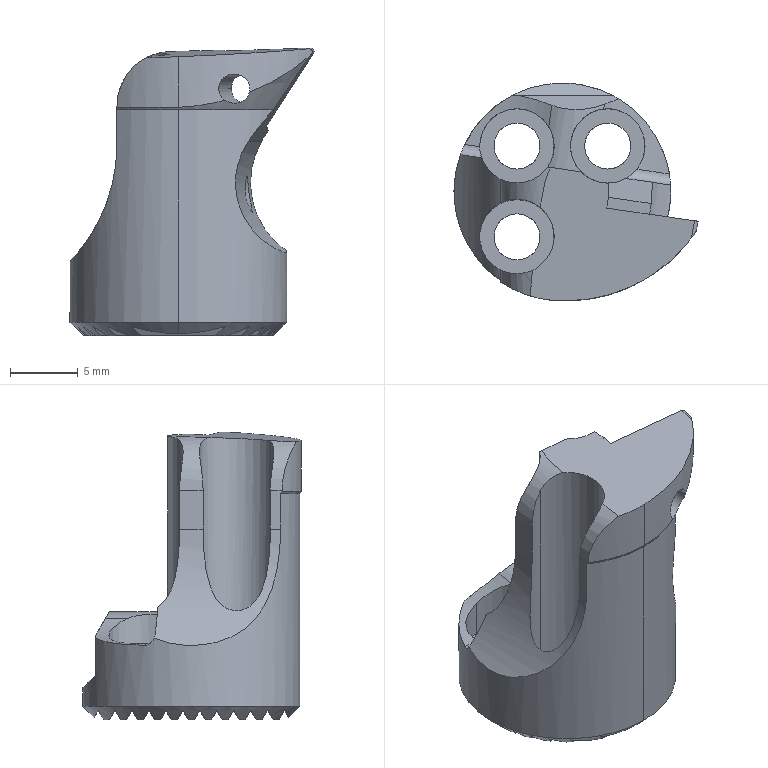Part | 1 solid | 129 faces | box 18.01 x 16.103 x 21.25 mm | volume 1797 mm3 | plane 88 | cylinder 34 | cone 5 | torus 2 | commonest cylinder face diameters 5.5 x7 3.4 x6 2 x2 2.16 x2 3.5 x2 4 x2